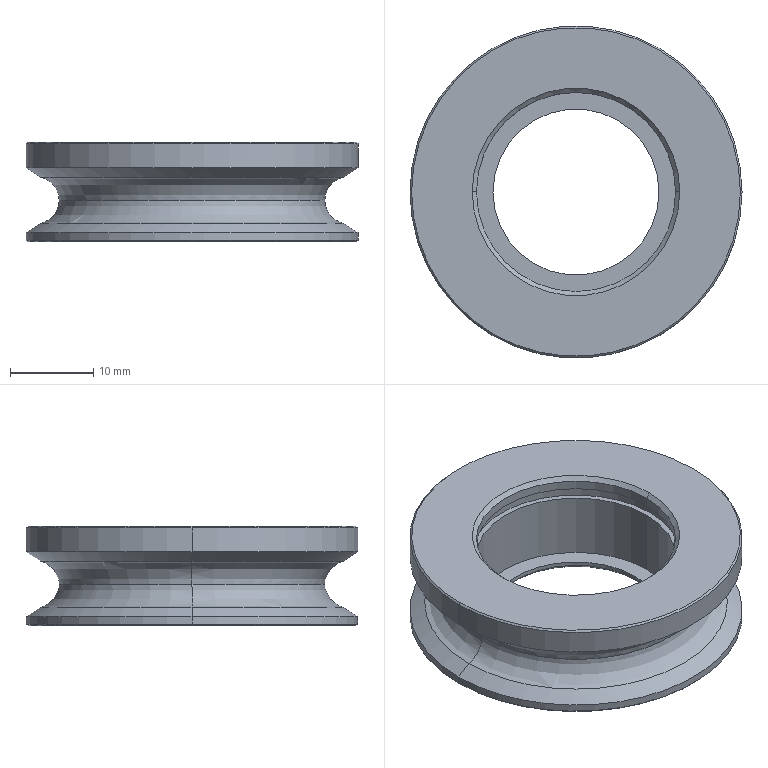Part | STEP file | 10000020541swp000-1 | 1 solid | 33 faces | box 40 x 40 x 12 mm | volume 7266 mm3 | cylinder 12 | cone 12 | plane 5 | torus 4 | commonest cylinder face diameters 24 x4 40 x4 20 x2 25.3 x2
STEP:
#1=CARTESIAN_POINT('',(12.65,0.,10.4));
#2=VERTEX_POINT('',#1);
#3=CARTESIAN_POINT('',(-12.65,0.,10.4));
#4=VERTEX_POINT('',#3);
#5=CARTESIAN_POINT('',(0.,0.,10.4));
#6=DIRECTION('',(0.,0.,-1.));
#7=DIRECTION('',(-1.,0.,0.));
#8=AXIS2_PLACEMENT_3D('',#5,#6,#7);
#9=CIRCLE('',#8,12.65);
#10=EDGE_CURVE('',#2,#4,#9,.T.);
#11=ORIENTED_EDGE('',*,*,#10,.F.);
#12=CARTESIAN_POINT('',(12.65,0.,9.));
#13=VERTEX_POINT('',#12);
#14=CARTESIAN_POINT('',(12.65,0.,0.));
#15=DIRECTION('',(0.,0.,-1.));
#16=VECTOR('',#15,1000.);
#17=LINE('',#14,#16);
#18=EDGE_CURVE('',#2,#13,#17,.T.);
#19=ORIENTED_EDGE('',*,*,#18,.T.);
#20=CARTESIAN_POINT('',(-12.65,0.,9.));
#21=VERTEX_POINT('',#20);
#22=CARTESIAN_POINT('',(0.,0.,9.));
#23=DIRECTION('',(0.,0.,-1.));
#24=DIRECTION('',(-1.,0.,0.));
#25=AXIS2_PLACEMENT_3D('',#22,#23,#24);
#26=CIRCLE('',#25,12.65);
#27=EDGE_CURVE('',#13,#21,#26,.T.);
#28=ORIENTED_EDGE('',*,*,#27,.T.);
#29=CARTESIAN_POINT('',(-12.65,0.,0.));
#30=DIRECTION('',(0.,0.,-1.));
#31=VECTOR('',#30,1000.);
#32=LINE('',#29,#31);
#33=EDGE_CURVE('',#4,#21,#32,.T.);
#34=ORIENTED_EDGE('',*,*,#33,.F.);
#35=EDGE_LOOP('',(#11,#19,#28,#34));
#36=FACE_OUTER_BOUND('',#35,.T.);
#37=CARTESIAN_POINT('',(0.,0.,0.));
#38=DIRECTION('',(0.,0.,-1.));
#39=DIRECTION('',(-1.,0.,0.));
#40=AXIS2_PLACEMENT_3D('',#37,#38,#39);
#41=CYLINDRICAL_SURFACE('',#40,12.65);
#42=ADVANCED_FACE('',(#36),#41,.F.);
#43=CARTESIAN_POINT('',(10.,0.,0.5));
#44=VERTEX_POINT('',#43);
#45=CARTESIAN_POINT('',(-10.,0.,0.5));
#46=VERTEX_POINT('',#45);
#47=CARTESIAN_POINT('',(0.,0.,0.5));
#48=DIRECTION('',(0.,0.,-1.));
#49=DIRECTION('',(1.,0.,0.));
#50=AXIS2_PLACEMENT_3D('',#47,#48,#49);
#51=CIRCLE('',#50,10.);
#52=EDGE_CURVE('',#44,#46,#51,.T.);
#53=ORIENTED_EDGE('',*,*,#52,.F.);
#54=CARTESIAN_POINT('',(10.5,0.,0.));
#55=VERTEX_POINT('',#54);
#56=CARTESIAN_POINT('',(10.5,0.,0.));
#57=DIRECTION('',(0.7071,0.,-0.7071));
#58=VECTOR('',#57,1000.);
#59=LINE('',#56,#58);
#60=EDGE_CURVE('',#44,#55,#59,.T.);
#61=ORIENTED_EDGE('',*,*,#60,.T.);
#62=CARTESIAN_POINT('',(-10.5,0.,0.));
#63=VERTEX_POINT('',#62);
#64=CARTESIAN_POINT('',(0.,0.,0.));
#65=DIRECTION('',(0.,0.,1.));
#66=DIRECTION('',(1.,0.,0.));
#67=AXIS2_PLACEMENT_3D('',#64,#65,#66);
#68=CIRCLE('',#67,10.5);
#69=EDGE_CURVE('',#63,#55,#68,.T.);
#70=ORIENTED_EDGE('',*,*,#69,.F.);
#71=CARTESIAN_POINT('',(-10.5,0.,0.));
#72=DIRECTION('',(-0.7071,0.,-0.7071));
#73=VECTOR('',#72,1000.);
#74=LINE('',#71,#73);
#75=EDGE_CURVE('',#46,#63,#74,.T.);
#76=ORIENTED_EDGE('',*,*,#75,.F.);
#77=EDGE_LOOP('',(#53,#61,#70,#76));
#78=FACE_OUTER_BOUND('',#77,.T.);
#79=CARTESIAN_POINT('',(0.,0.,0.));
#80=DIRECTION('',(0.,0.,-1.));
#81=DIRECTION('',(-1.,0.,0.));
#82=AXIS2_PLACEMENT_3D('',#79,#80,#81);
#83=CONICAL_SURFACE('',#82,10.5,0.7854);
#84=ADVANCED_FACE('',(#78),#83,.F.);
#85=CARTESIAN_POINT('',(-12.,0.,11.5));
#86=VERTEX_POINT('',#85);
#87=CARTESIAN_POINT('',(12.,0.,11.5));
#88=VERTEX_POINT('',#87);
#89=CARTESIAN_POINT('',(0.,0.,11.5));
#90=DIRECTION('',(0.,0.,1.));
#91=DIRECTION('',(1.,0.,0.));
#92=AXIS2_PLACEMENT_3D('',#89,#90,#91);
#93=CIRCLE('',#92,12.);
#94=EDGE_CURVE('',#86,#88,#93,.T.);
#95=ORIENTED_EDGE('',*,*,#94,.F.);
#96=CARTESIAN_POINT('',(-12.5,0.,12.));
#97=VERTEX_POINT('',#96);
#98=CARTESIAN_POINT('',(-12.,0.,11.5));
#99=DIRECTION('',(-0.7071,0.,0.7071));
#100=VECTOR('',#99,1000.);
#101=LINE('',#98,#100);
#102=EDGE_CURVE('',#86,#97,#101,.T.);
#103=ORIENTED_EDGE('',*,*,#102,.T.);
#104=CARTESIAN_POINT('',(12.5,0.,12.));
#105=VERTEX_POINT('',#104);
#106=CARTESIAN_POINT('',(0.,0.,12.));
#107=DIRECTION('',(0.,0.,-1.));
#108=DIRECTION('',(1.,0.,0.));
#109=AXIS2_PLACEMENT_3D('',#106,#107,#108);
#110=CIRCLE('',#109,12.5);
#111=EDGE_CURVE('',#105,#97,#110,.T.);
#112=ORIENTED_EDGE('',*,*,#111,.F.);
#113=CARTESIAN_POINT('',(12.,0.,11.5));
#114=DIRECTION('',(0.7071,0.,0.7071));
#115=VECTOR('',#114,1000.);
#116=LINE('',#113,#115);
#117=EDGE_CURVE('',#88,#105,#116,.T.);
#118=ORIENTED_EDGE('',*,*,#117,.F.);
#119=EDGE_LOOP('',(#95,#103,#112,#118));
#120=FACE_OUTER_BOUND('',#119,.T.);
#121=CARTESIAN_POINT('',(0.,0.,11.5));
#122=DIRECTION('',(0.,0.,1.));
#123=DIRECTION('',(1.,0.,0.));
#124=AXIS2_PLACEMENT_3D('',#121,#122,#123);
#125=CONICAL_SURFACE('',#124,12.,0.7854);
#126=ADVANCED_FACE('',(#120),#125,.F.);
#127=CARTESIAN_POINT('',(-19.8,0.,0.));
#128=VERTEX_POINT('',#127);
#129=CARTESIAN_POINT('',(19.8,0.,0.));
#130=VERTEX_POINT('',#129);
#131=CARTESIAN_POINT('',(0.,0.,0.));
#132=DIRECTION('',(0.,0.,-1.));
#133=DIRECTION('',(1.,0.,0.));
#134=AXIS2_PLACEMENT_3D('',#131,#132,#133);
#135=CIRCLE('',#134,19.8);
#136=EDGE_CURVE('',#128,#130,#135,.T.);
#137=ORIENTED_EDGE('',*,*,#136,.F.);
#138=CARTESIAN_POINT('',(-20.,0.,0.2));
#139=VERTEX_POINT('',#138);
#140=CARTESIAN_POINT('',(-20.,0.,0.2));
#141=DIRECTION('',(-0.7071,0.,0.7071));
#142=VECTOR('',#141,1000.);
#143=LINE('',#140,#142);
#144=EDGE_CURVE('',#128,#139,#143,.T.);
#145=ORIENTED_EDGE('',*,*,#144,.T.);
#146=CARTESIAN_POINT('',(20.,0.,0.2));
#147=VERTEX_POINT('',#146);
#148=CARTESIAN_POINT('',(0.,0.,0.2));
#149=DIRECTION('',(0.,0.,1.));
#150=DIRECTION('',(1.,0.,0.));
#151=AXIS2_PLACEMENT_3D('',#148,#149,#150);
#152=CIRCLE('',#151,20.);
#153=EDGE_CURVE('',#147,#139,#152,.T.);
#154=ORIENTED_EDGE('',*,*,#153,.F.);
#155=CARTESIAN_POINT('',(20.,0.,0.2));
#156=DIRECTION('',(0.7071,0.,0.7071));
#157=VECTOR('',#156,1000.);
#158=LINE('',#155,#157);
#159=EDGE_CURVE('',#130,#147,#158,.T.);
#160=ORIENTED_EDGE('',*,*,#159,.F.);
#161=EDGE_LOOP('',(#137,#145,#154,#160));
#162=FACE_OUTER_BOUND('',#161,.T.);
#163=CARTESIAN_POINT('',(0.,0.,0.2));
#164=DIRECTION('',(0.,0.,1.));
#165=DIRECTION('',(1.,0.,0.));
#166=AXIS2_PLACEMENT_3D('',#163,#164,#165);
#167=CONICAL_SURFACE('',#166,20.,0.7854);
#168=ADVANCED_FACE('',(#162),#167,.T.);
#169=CARTESIAN_POINT('',(19.8,0.,12.));
#170=VERTEX_POINT('',#169);
#171=CARTESIAN_POINT('',(-19.8,0.,12.));
#172=VERTEX_POINT('',#171);
#173=CARTESIAN_POINT('',(0.,0.,12.));
#174=DIRECTION('',(0.,0.,1.));
#175=DIRECTION('',(1.,0.,0.));
#176=AXIS2_PLACEMENT_3D('',#173,#174,#175);
#177=CIRCLE('',#176,19.8);
#178=EDGE_CURVE('',#170,#172,#177,.T.);
#179=ORIENTED_EDGE('',*,*,#178,.F.);
#180=CARTESIAN_POINT('',(20.,0.,11.8));
#181=VERTEX_POINT('',#180);
#182=CARTESIAN_POINT('',(19.8,0.,12.));
#183=DIRECTION('',(0.7071,0.,-0.7071));
#184=VECTOR('',#183,1000.);
#185=LINE('',#182,#184);
#186=EDGE_CURVE('',#170,#181,#185,.T.);
#187=ORIENTED_EDGE('',*,*,#186,.T.);
#188=CARTESIAN_POINT('',(-20.,0.,11.8));
#189=VERTEX_POINT('',#188);
#190=CARTESIAN_POINT('',(0.,0.,11.8));
#191=DIRECTION('',(0.,0.,-1.));
#192=DIRECTION('',(1.,0.,0.));
#193=AXIS2_PLACEMENT_3D('',#190,#191,#192);
#194=CIRCLE('',#193,20.);
#195=EDGE_CURVE('',#189,#181,#194,.T.);
#196=ORIENTED_EDGE('',*,*,#195,.F.);
#197=CARTESIAN_POINT('',(-19.8,0.,12.));
#198=DIRECTION('',(-0.7071,0.,-0.7071));
#199=VECTOR('',#198,1000.);
#200=LINE('',#197,#199);
#201=EDGE_CURVE('',#172,#189,#200,.T.);
#202=ORIENTED_EDGE('',*,*,#201,.F.);
#203=EDGE_LOOP('',(#179,#187,#196,#202));
#204=FACE_OUTER_BOUND('',#203,.T.);
#205=CARTESIAN_POINT('',(0.,0.,12.));
#206=DIRECTION('',(0.,0.,-1.));
#207=DIRECTION('',(-1.,0.,0.));
#208=AXIS2_PLACEMENT_3D('',#205,#206,#207);
#209=CONICAL_SURFACE('',#208,19.8,0.7854);
#210=ADVANCED_FACE('',(#204),#209,.T.);
#211=CARTESIAN_POINT('',(-18.244,0.,7.785));
#212=VERTEX_POINT('',#211);
#213=CARTESIAN_POINT('',(18.244,0.,7.785));
#214=VERTEX_POINT('',#213);
#215=CARTESIAN_POINT('',(0.,0.,7.785));
#216=DIRECTION('',(0.,0.,-1.));
#217=DIRECTION('',(-1.,0.,0.));
#218=AXIS2_PLACEMENT_3D('',#215,#216,#217);
#219=CIRCLE('',#218,18.244);
#220=EDGE_CURVE('',#212,#214,#219,.T.);
#221=ORIENTED_EDGE('',*,*,#220,.F.);
#222=CARTESIAN_POINT('',(-20.,0.,8.909));
#223=VERTEX_POINT('',#222);
#224=CARTESIAN_POINT('',(-20.,0.,8.909));
#225=DIRECTION('',(-0.8422,0.,0.5391));
#226=VECTOR('',#225,1000.);
#227=LINE('',#224,#226);
#228=EDGE_CURVE('',#212,#223,#227,.T.);
#229=ORIENTED_EDGE('',*,*,#228,.T.);
#230=CARTESIAN_POINT('',(20.,0.,8.909));
#231=VERTEX_POINT('',#230);
#232=CARTESIAN_POINT('',(0.,0.,8.909));
#233=DIRECTION('',(0.,0.,1.));
#234=DIRECTION('',(1.,0.,0.));
#235=AXIS2_PLACEMENT_3D('',#232,#233,#234);
#236=CIRCLE('',#235,20.);
#237=EDGE_CURVE('',#231,#223,#236,.T.);
#238=ORIENTED_EDGE('',*,*,#237,.F.);
#239=CARTESIAN_POINT('',(20.,0.,8.909));
#240=DIRECTION('',(0.8422,0.,0.5391));
#241=VECTOR('',#240,1000.);
#242=LINE('',#239,#241);
#243=EDGE_CURVE('',#214,#231,#242,.T.);
#244=ORIENTED_EDGE('',*,*,#243,.F.);
#245=EDGE_LOOP('',(#221,#229,#238,#244));
#246=FACE_OUTER_BOUND('',#245,.T.);
#247=CARTESIAN_POINT('',(0.,0.,8.909));
#248=DIRECTION('',(0.,0.,1.));
#249=DIRECTION('',(1.,0.,0.));
#250=AXIS2_PLACEMENT_3D('',#247,#248,#249);
#251=CONICAL_SURFACE('',#250,20.,1.001);
#252=ADVANCED_FACE('',(#246),#251,.T.);
#253=CARTESIAN_POINT('',(18.244,0.,2.215));
#254=VERTEX_POINT('',#253);
#255=CARTESIAN_POINT('',(-18.244,0.,2.215));
#256=VERTEX_POINT('',#255);
#257=CARTESIAN_POINT('',(0.,0.,2.215));
#258=DIRECTION('',(0.,0.,1.));
#259=DIRECTION('',(1.,0.,0.));
#260=AXIS2_PLACEMENT_3D('',#257,#258,#259);
#261=CIRCLE('',#260,18.244);
#262=EDGE_CURVE('',#254,#256,#261,.T.);
#263=ORIENTED_EDGE('',*,*,#262,.F.);
#264=CARTESIAN_POINT('',(20.,0.,1.091));
#265=VERTEX_POINT('',#264);
#266=CARTESIAN_POINT('',(18.244,0.,2.215));
#267=DIRECTION('',(0.8422,0.,-0.5391));
#268=VECTOR('',#267,1000.);
#269=LINE('',#266,#268);
#270=EDGE_CURVE('',#254,#265,#269,.T.);
#271=ORIENTED_EDGE('',*,*,#270,.T.);
#272=CARTESIAN_POINT('',(-20.,0.,1.091));
#273=VERTEX_POINT('',#272);
#274=CARTESIAN_POINT('',(0.,0.,1.091));
#275=DIRECTION('',(0.,0.,-1.));
#276=DIRECTION('',(-1.,0.,0.));
#277=AXIS2_PLACEMENT_3D('',#274,#275,#276);
#278=CIRCLE('',#277,20.);
#279=EDGE_CURVE('',#273,#265,#278,.T.);
#280=ORIENTED_EDGE('',*,*,#279,.F.);
#281=CARTESIAN_POINT('',(-18.244,0.,2.215));
#282=DIRECTION('',(-0.8422,0.,-0.5391));
#283=VECTOR('',#282,1000.);
#284=LINE('',#281,#283);
#285=EDGE_CURVE('',#256,#273,#284,.T.);
#286=ORIENTED_EDGE('',*,*,#285,.F.);
#287=EDGE_LOOP('',(#263,#271,#280,#286));
#288=FACE_OUTER_BOUND('',#287,.T.);
#289=CARTESIAN_POINT('',(0.,0.,2.215));
#290=DIRECTION('',(0.,0.,-1.));
#291=DIRECTION('',(-1.,0.,0.));
#292=AXIS2_PLACEMENT_3D('',#289,#290,#291);
#293=CONICAL_SURFACE('',#292,18.244,1.001);
#294=ADVANCED_FACE('',(#288),#293,.T.);
#295=CARTESIAN_POINT('',(0.,0.,2.215));
#296=DIRECTION('',(0.,0.,1.));
#297=DIRECTION('',(1.,0.,0.));
#298=AXIS2_PLACEMENT_3D('',#295,#296,#297);
#299=CIRCLE('',#298,18.244);
#300=EDGE_CURVE('',#256,#254,#299,.T.);
#301=ORIENTED_EDGE('',*,*,#300,.T.);
#302=CARTESIAN_POINT('',(16.,0.,5.));
#303=VERTEX_POINT('',#302);
#304=CARTESIAN_POINT('',(18.85,0.,5.));
#305=DIRECTION('',(0.,1.,0.));
#306=DIRECTION('',(-1.,0.,0.));
#307=AXIS2_PLACEMENT_3D('',#304,#305,#306);
#308=CIRCLE('',#307,2.85);
#309=EDGE_CURVE('',#254,#303,#308,.T.);
#310=ORIENTED_EDGE('',*,*,#309,.T.);
#311=CARTESIAN_POINT('',(-16.,0.,5.));
#312=VERTEX_POINT('',#311);
#313=CARTESIAN_POINT('',(0.,0.,5.));
#314=DIRECTION('',(0.,0.,-1.));
#315=DIRECTION('',(1.,0.,0.));
#316=AXIS2_PLACEMENT_3D('',#313,#314,#315);
#317=CIRCLE('',#316,16.);
#318=EDGE_CURVE('',#303,#312,#317,.T.);
#319=ORIENTED_EDGE('',*,*,#318,.T.);
#320=CARTESIAN_POINT('',(-18.85,0.,5.));
#321=DIRECTION('',(0.,-1.,0.));
#322=DIRECTION('',(0.,0.,-1.));
#323=AXIS2_PLACEMENT_3D('',#320,#321,#322);
#324=CIRCLE('',#323,2.85);
#325=EDGE_CURVE('',#256,#312,#324,.T.);
#326=ORIENTED_EDGE('',*,*,#325,.F.);
#327=EDGE_LOOP('',(#301,#310,#319,#326));
#328=FACE_OUTER_BOUND('',#327,.T.);
#329=CARTESIAN_POINT('',(0.,0.,5.));
#330=DIRECTION('',(0.,0.,-1.));
#331=DIRECTION('',(-1.,0.,0.));
#332=AXIS2_PLACEMENT_3D('',#329,#330,#331);
#333=TOROIDAL_SURFACE('',#332,18.85,2.85);
#334=ADVANCED_FACE('',(#328),#333,.F.);
#335=CARTESIAN_POINT('',(0.,0.,7.785));
#336=DIRECTION('',(0.,0.,-1.));
#337=DIRECTION('',(-1.,0.,0.));
#338=AXIS2_PLACEMENT_3D('',#335,#336,#337);
#339=CIRCLE('',#338,18.244);
#340=EDGE_CURVE('',#214,#212,#339,.T.);
#341=ORIENTED_EDGE('',*,*,#340,.T.);
#342=CARTESIAN_POINT('',(-18.85,0.,5.));
#343=DIRECTION('',(0.,1.,0.));
#344=DIRECTION('',(-1.,0.,0.));
#345=AXIS2_PLACEMENT_3D('',#342,#343,#344);
#346=CIRCLE('',#345,2.85);
#347=EDGE_CURVE('',#212,#312,#346,.T.);
#348=ORIENTED_EDGE('',*,*,#347,.T.);
#349=ORIENTED_EDGE('',*,*,#318,.F.);
#350=CARTESIAN_POINT('',(18.85,0.,5.));
#351=DIRECTION('',(0.,-1.,0.));
#352=DIRECTION('',(0.,0.,-1.));
#353=AXIS2_PLACEMENT_3D('',#350,#351,#352);
#354=CIRCLE('',#353,2.85);
#355=EDGE_CURVE('',#214,#303,#354,.T.);
#356=ORIENTED_EDGE('',*,*,#355,.F.);
#357=EDGE_LOOP('',(#341,#348,#349,#356));
#358=FACE_OUTER_BOUND('',#357,.T.);
#359=CARTESIAN_POINT('',(0.,0.,5.));
#360=DIRECTION('',(0.,0.,1.));
#361=DIRECTION('',(1.,0.,0.));
#362=AXIS2_PLACEMENT_3D('',#359,#360,#361);
#363=TOROIDAL_SURFACE('',#362,18.85,2.85);
#364=ADVANCED_FACE('',(#358),#363,.F.);
#365=CARTESIAN_POINT('',(-12.,0.,1.));
#366=VERTEX_POINT('',#365);
#367=CARTESIAN_POINT('',(12.,0.,1.));
#368=VERTEX_POINT('',#367);
#369=CARTESIAN_POINT('',(0.,0.,1.));
#370=DIRECTION('',(0.,0.,1.));
#371=DIRECTION('',(1.,0.,0.));
#372=AXIS2_PLACEMENT_3D('',#369,#370,#371);
#373=CIRCLE('',#372,12.);
#374=EDGE_CURVE('',#366,#368,#373,.T.);
#375=ORIENTED_EDGE('',*,*,#374,.F.);
#376=CARTESIAN_POINT('',(-12.,0.,9.));
#377=VERTEX_POINT('',#376);
#378=CARTESIAN_POINT('',(-12.,0.,1.));
#379=DIRECTION('',(0.,0.,1.));
#380=VECTOR('',#379,1000.);
#381=LINE('',#378,#380);
#382=EDGE_CURVE('',#366,#377,#381,.T.);
#383=ORIENTED_EDGE('',*,*,#382,.T.);
#384=CARTESIAN_POINT('',(12.,0.,9.));
#385=VERTEX_POINT('',#384);
#386=CARTESIAN_POINT('',(0.,0.,9.));
#387=DIRECTION('',(0.,0.,1.));
#388=DIRECTION('',(-1.,0.,0.));
#389=AXIS2_PLACEMENT_3D('',#386,#387,#388);
#390=CIRCLE('',#389,12.);
#391=EDGE_CURVE('',#377,#385,#390,.T.);
#392=ORIENTED_EDGE('',*,*,#391,.T.);
#393=CARTESIAN_POINT('',(12.,0.,1.));
#394=DIRECTION('',(0.,0.,1.));
#395=VECTOR('',#394,1000.);
#396=LINE('',#393,#395);
#397=EDGE_CURVE('',#368,#385,#396,.T.);
#398=ORIENTED_EDGE('',*,*,#397,.F.);
#399=EDGE_LOOP('',(#375,#383,#392,#398));
#400=FACE_OUTER_BOUND('',#399,.T.);
#401=CARTESIAN_POINT('',(0.,0.,1.));
#402=DIRECTION('',(0.,0.,1.));
#403=DIRECTION('',(1.,0.,0.));
#404=AXIS2_PLACEMENT_3D('',#401,#402,#403);
#405=CYLINDRICAL_SURFACE('',#404,12.);
#406=ADVANCED_FACE('',(#400),#405,.F.);
#407=ORIENTED_EDGE('',*,*,#279,.T.);
#408=CARTESIAN_POINT('',(20.,0.,12.));
#409=DIRECTION('',(0.,0.,-1.));
#410=VECTOR('',#409,1000.);
#411=LINE('',#408,#410);
#412=EDGE_CURVE('',#265,#147,#411,.T.);
#413=ORIENTED_EDGE('',*,*,#412,.T.);
#414=ORIENTED_EDGE('',*,*,#153,.T.);
#415=CARTESIAN_POINT('',(-20.,0.,12.));
#416=DIRECTION('',(0.,0.,-1.));
#417=VECTOR('',#416,1000.);
#418=LINE('',#415,#417);
#419=EDGE_CURVE('',#273,#139,#418,.T.);
#420=ORIENTED_EDGE('',*,*,#419,.F.);
#421=EDGE_LOOP('',(#407,#413,#414,#420));
#422=FACE_OUTER_BOUND('',#421,.T.);
#423=CARTESIAN_POINT('',(0.,0.,12.));
#424=DIRECTION('',(0.,0.,-1.));
#425=DIRECTION('',(-1.,0.,0.));
#426=AXIS2_PLACEMENT_3D('',#423,#424,#425);
#427=CYLINDRICAL_SURFACE('',#426,20.);
#428=ADVANCED_FACE('',(#422),#427,.T.);
#429=ORIENTED_EDGE('',*,*,#195,.T.);
#430=CARTESIAN_POINT('',(20.,0.,12.));
#431=DIRECTION('',(0.,0.,-1.));
#432=VECTOR('',#431,1000.);
#433=LINE('',#430,#432);
#434=EDGE_CURVE('',#181,#231,#433,.T.);
#435=ORIENTED_EDGE('',*,*,#434,.T.);
#436=ORIENTED_EDGE('',*,*,#237,.T.);
#437=CARTESIAN_POINT('',(-20.,0.,12.));
#438=DIRECTION('',(0.,0.,-1.));
#439=VECTOR('',#438,1000.);
#440=LINE('',#437,#439);
#441=EDGE_CURVE('',#189,#223,#440,.T.);
#442=ORIENTED_EDGE('',*,*,#441,.F.);
#443=EDGE_LOOP('',(#429,#435,#436,#442));
#444=FACE_OUTER_BOUND('',#443,.T.);
#445=CARTESIAN_POINT('',(0.,0.,12.));
#446=DIRECTION('',(0.,0.,-1.));
#447=DIRECTION('',(-1.,0.,0.));
#448=AXIS2_PLACEMENT_3D('',#445,#446,#447);
#449=CYLINDRICAL_SURFACE('',#448,20.);
#450=ADVANCED_FACE('',(#444),#449,.T.);
#451=ORIENTED_EDGE('',*,*,#52,.T.);
#452=CARTESIAN_POINT('',(-10.,0.,1.));
#453=VERTEX_POINT('',#452);
#454=CARTESIAN_POINT('',(-10.,0.,12.));
#455=DIRECTION('',(0.,0.,1.));
#456=VECTOR('',#455,1000.);
#457=LINE('',#454,#456);
#458=EDGE_CURVE('',#46,#453,#457,.T.);
#459=ORIENTED_EDGE('',*,*,#458,.T.);
#460=CARTESIAN_POINT('',(10.,0.,1.));
#461=VERTEX_POINT('',#460);
#462=CARTESIAN_POINT('',(0.,0.,1.));
#463=DIRECTION('',(0.,0.,-1.));
#464=DIRECTION('',(1.,0.,0.));
#465=AXIS2_PLACEMENT_3D('',#462,#463,#464);
#466=CIRCLE('',#465,10.);
#467=EDGE_CURVE('',#461,#453,#466,.T.);
#468=ORIENTED_EDGE('',*,*,#467,.F.);
#469=CARTESIAN_POINT('',(10.,0.,12.));
#470=DIRECTION('',(0.,0.,1.));
#471=VECTOR('',#470,1000.);
#472=LINE('',#469,#471);
#473=EDGE_CURVE('',#44,#461,#472,.T.);
#474=ORIENTED_EDGE('',*,*,#473,.F.);
#475=EDGE_LOOP('',(#451,#459,#468,#474));
#476=FACE_OUTER_BOUND('',#475,.T.);
#477=CARTESIAN_POINT('',(0.,0.,12.));
#478=DIRECTION('',(0.,0.,1.));
#479=DIRECTION('',(1.,0.,0.));
#480=AXIS2_PLACEMENT_3D('',#477,#478,#479);
#481=CYLINDRICAL_SURFACE('',#480,10.);
#482=ADVANCED_FACE('',(#476),#481,.F.);
#483=CARTESIAN_POINT('',(12.,0.,10.4));
#484=VERTEX_POINT('',#483);
#485=CARTESIAN_POINT('',(-12.,0.,10.4));
#486=VERTEX_POINT('',#485);
#487=CARTESIAN_POINT('',(0.,0.,10.4));
#488=DIRECTION('',(0.,0.,-1.));
#489=DIRECTION('',(1.,0.,0.));
#490=AXIS2_PLACEMENT_3D('',#487,#488,#489);
#491=CIRCLE('',#490,12.);
#492=EDGE_CURVE('',#484,#486,#491,.T.);
#493=ORIENTED_EDGE('',*,*,#492,.T.);
#494=CARTESIAN_POINT('',(-12.,0.,1.));
#495=DIRECTION('',(0.,0.,1.));
#496=VECTOR('',#495,1000.);
#497=LINE('',#494,#496);
#498=EDGE_CURVE('',#486,#86,#497,.T.);
#499=ORIENTED_EDGE('',*,*,#498,.T.);
#500=ORIENTED_EDGE('',*,*,#94,.T.);
#501=CARTESIAN_POINT('',(12.,0.,1.));
#502=DIRECTION('',(0.,0.,1.));
#503=VECTOR('',#502,1000.);
#504=LINE('',#501,#503);
#505=EDGE_CURVE('',#484,#88,#504,.T.);
#506=ORIENTED_EDGE('',*,*,#505,.F.);
#507=EDGE_LOOP('',(#493,#499,#500,#506));
#508=FACE_OUTER_BOUND('',#507,.T.);
#509=CARTESIAN_POINT('',(0.,0.,1.));
#510=DIRECTION('',(0.,0.,1.));
#511=DIRECTION('',(1.,0.,0.));
#512=AXIS2_PLACEMENT_3D('',#509,#510,#511);
#513=CYLINDRICAL_SURFACE('',#512,12.);
#514=ADVANCED_FACE('',(#508),#513,.F.);
#515=ORIENTED_EDGE('',*,*,#498,.F.);
#516=CARTESIAN_POINT('',(0.,0.,10.4));
#517=DIRECTION('',(0.,0.,-1.));
#518=DIRECTION('',(1.,0.,0.));
#519=AXIS2_PLACEMENT_3D('',#516,#517,#518);
#520=CIRCLE('',#519,12.);
#521=EDGE_CURVE('',#486,#484,#520,.T.);
#522=ORIENTED_EDGE('',*,*,#521,.T.);
#523=ORIENTED_EDGE('',*,*,#505,.T.);
#524=CARTESIAN_POINT('',(0.,0.,11.5));
#525=DIRECTION('',(0.,0.,1.));
#526=DIRECTION('',(1.,0.,0.));
#527=AXIS2_PLACEMENT_3D('',#524,#525,#526);
#528=CIRCLE('',#527,12.);
#529=EDGE_CURVE('',#88,#86,#528,.T.);
#530=ORIENTED_EDGE('',*,*,#529,.T.);
#531=EDGE_LOOP('',(#515,#522,#523,#530));
#532=FACE_OUTER_BOUND('',#531,.T.);
#533=CARTESIAN_POINT('',(0.,0.,1.));
#534=DIRECTION('',(0.,0.,1.));
#535=DIRECTION('',(1.,0.,0.));
#536=AXIS2_PLACEMENT_3D('',#533,#534,#535);
#537=CYLINDRICAL_SURFACE('',#536,12.);
#538=ADVANCED_FACE('',(#532),#537,.F.);
#539=ORIENTED_EDGE('',*,*,#458,.F.);
#540=CARTESIAN_POINT('',(0.,0.,0.5));
#541=DIRECTION('',(0.,0.,-1.));
#542=DIRECTION('',(1.,0.,0.));
#543=AXIS2_PLACEMENT_3D('',#540,#541,#542);
#544=CIRCLE('',#543,10.);
#545=EDGE_CURVE('',#46,#44,#544,.T.);
#546=ORIENTED_EDGE('',*,*,#545,.T.);
#547=ORIENTED_EDGE('',*,*,#473,.T.);
#548=CARTESIAN_POINT('',(0.,0.,1.));
#549=DIRECTION('',(0.,0.,-1.));
#550=DIRECTION('',(1.,0.,0.));
#551=AXIS2_PLACEMENT_3D('',#548,#549,#550);
#552=CIRCLE('',#551,10.);
#553=EDGE_CURVE('',#453,#461,#552,.T.);
#554=ORIENTED_EDGE('',*,*,#553,.F.);
#555=EDGE_LOOP('',(#539,#546,#547,#554));
#556=FACE_OUTER_BOUND('',#555,.T.);
#557=CARTESIAN_POINT('',(0.,0.,12.));
#558=DIRECTION('',(0.,0.,1.));
#559=DIRECTION('',(1.,0.,0.));
#560=AXIS2_PLACEMENT_3D('',#557,#558,#559);
#561=CYLINDRICAL_SURFACE('',#560,10.);
#562=ADVANCED_FACE('',(#556),#561,.F.);
#563=ORIENTED_EDGE('',*,*,#434,.F.);
#564=CARTESIAN_POINT('',(0.,0.,11.8));
#565=DIRECTION('',(0.,0.,-1.));
#566=DIRECTION('',(1.,0.,0.));
#567=AXIS2_PLACEMENT_3D('',#564,#565,#566);
#568=CIRCLE('',#567,20.);
#569=EDGE_CURVE('',#181,#189,#568,.T.);
#570=ORIENTED_EDGE('',*,*,#569,.T.);
#571=ORIENTED_EDGE('',*,*,#441,.T.);
#572=CARTESIAN_POINT('',(0.,0.,8.909));
#573=DIRECTION('',(0.,0.,1.));
#574=DIRECTION('',(1.,0.,0.));
#575=AXIS2_PLACEMENT_3D('',#572,#573,#574);
#576=CIRCLE('',#575,20.);
#577=EDGE_CURVE('',#223,#231,#576,.T.);
#578=ORIENTED_EDGE('',*,*,#577,.T.);
#579=EDGE_LOOP('',(#563,#570,#571,#578));
#580=FACE_OUTER_BOUND('',#579,.T.);
#581=CARTESIAN_POINT('',(0.,0.,12.));
#582=DIRECTION('',(0.,0.,-1.));
#583=DIRECTION('',(-1.,0.,0.));
#584=AXIS2_PLACEMENT_3D('',#581,#582,#583);
#585=CYLINDRICAL_SURFACE('',#584,20.);
#586=ADVANCED_FACE('',(#580),#585,.T.);
#587=ORIENTED_EDGE('',*,*,#412,.F.);
#588=CARTESIAN_POINT('',(0.,0.,1.091));
#589=DIRECTION('',(0.,0.,-1.));
#590=DIRECTION('',(-1.,0.,0.));
#591=AXIS2_PLACEMENT_3D('',#588,#589,#590);
#592=CIRCLE('',#591,20.);
#593=EDGE_CURVE('',#265,#273,#592,.T.);
#594=ORIENTED_EDGE('',*,*,#593,.T.);
#595=ORIENTED_EDGE('',*,*,#419,.T.);
#596=CARTESIAN_POINT('',(0.,0.,0.2));
#597=DIRECTION('',(0.,0.,1.));
#598=DIRECTION('',(1.,0.,0.));
#599=AXIS2_PLACEMENT_3D('',#596,#597,#598);
#600=CIRCLE('',#599,20.);
#601=EDGE_CURVE('',#139,#147,#600,.T.);
#602=ORIENTED_EDGE('',*,*,#601,.T.);
#603=EDGE_LOOP('',(#587,#594,#595,#602));
#604=FACE_OUTER_BOUND('',#603,.T.);
#605=CARTESIAN_POINT('',(0.,0.,12.));
#606=DIRECTION('',(0.,0.,-1.));
#607=DIRECTION('',(-1.,0.,0.));
#608=AXIS2_PLACEMENT_3D('',#605,#606,#607);
#609=CYLINDRICAL_SURFACE('',#608,20.);
#610=ADVANCED_FACE('',(#604),#609,.T.);
#611=ORIENTED_EDGE('',*,*,#111,.T.);
#612=CARTESIAN_POINT('',(0.,0.,12.));
#613=DIRECTION('',(0.,0.,-1.));
#614=DIRECTION('',(1.,0.,0.));
#615=AXIS2_PLACEMENT_3D('',#612,#613,#614);
#616=CIRCLE('',#615,12.5);
#617=EDGE_CURVE('',#97,#105,#616,.T.);
#618=ORIENTED_EDGE('',*,*,#617,.T.);
#619=EDGE_LOOP('',(#611,#618));
#620=FACE_BOUND('',#619,.T.);
#621=CARTESIAN_POINT('',(0.,0.,12.));
#622=DIRECTION('',(0.,0.,1.));
#623=DIRECTION('',(1.,0.,0.));
#624=AXIS2_PLACEMENT_3D('',#621,#622,#623);
#625=CIRCLE('',#624,19.8);
#626=EDGE_CURVE('',#172,#170,#625,.T.);
#627=ORIENTED_EDGE('',*,*,#626,.T.);
#628=ORIENTED_EDGE('',*,*,#178,.T.);
#629=EDGE_LOOP('',(#627,#628));
#630=FACE_OUTER_BOUND('',#629,.T.);
#631=CARTESIAN_POINT('',(0.,0.,12.));
#632=DIRECTION('',(0.,0.,1.));
#633=DIRECTION('',(1.,0.,0.));
#634=AXIS2_PLACEMENT_3D('',#631,#632,#633);
#635=PLANE('',#634);
#636=ADVANCED_FACE('',(#620,#630),#635,.T.);
#637=ORIENTED_EDGE('',*,*,#69,.T.);
#638=CARTESIAN_POINT('',(0.,0.,0.));
#639=DIRECTION('',(0.,0.,1.));
#640=DIRECTION('',(1.,0.,0.));
#641=AXIS2_PLACEMENT_3D('',#638,#639,#640);
#642=CIRCLE('',#641,10.5);
#643=EDGE_CURVE('',#55,#63,#642,.T.);
#644=ORIENTED_EDGE('',*,*,#643,.T.);
#645=EDGE_LOOP('',(#637,#644));
#646=FACE_BOUND('',#645,.T.);
#647=CARTESIAN_POINT('',(0.,0.,0.));
#648=DIRECTION('',(0.,0.,-1.));
#649=DIRECTION('',(1.,0.,0.));
#650=AXIS2_PLACEMENT_3D('',#647,#648,#649);
#651=CIRCLE('',#650,19.8);
#652=EDGE_CURVE('',#130,#128,#651,.T.);
#653=ORIENTED_EDGE('',*,*,#652,.T.);
#654=ORIENTED_EDGE('',*,*,#136,.T.);
#655=EDGE_LOOP('',(#653,#654));
#656=FACE_OUTER_BOUND('',#655,.T.);
#657=CARTESIAN_POINT('',(0.,0.,0.));
#658=DIRECTION('',(0.,0.,1.));
#659=DIRECTION('',(1.,0.,0.));
#660=AXIS2_PLACEMENT_3D('',#657,#658,#659);
#661=PLANE('',#660);
#662=ADVANCED_FACE('',(#646,#656),#661,.F.);
#663=CARTESIAN_POINT('',(0.,0.,1.));
#664=DIRECTION('',(0.,0.,1.));
#665=DIRECTION('',(1.,0.,0.));
#666=AXIS2_PLACEMENT_3D('',#663,#664,#665);
#667=CIRCLE('',#666,12.);
#668=EDGE_CURVE('',#368,#366,#667,.T.);
#669=ORIENTED_EDGE('',*,*,#668,.T.);
#670=ORIENTED_EDGE('',*,*,#374,.T.);
#671=EDGE_LOOP('',(#669,#670));
#672=FACE_OUTER_BOUND('',#671,.T.);
#673=ORIENTED_EDGE('',*,*,#467,.T.);
#674=ORIENTED_EDGE('',*,*,#553,.T.);
#675=EDGE_LOOP('',(#673,#674));
#676=FACE_BOUND('',#675,.T.);
#677=CARTESIAN_POINT('',(0.,0.,1.));
#678=DIRECTION('',(0.,0.,1.));
#679=DIRECTION('',(1.,0.,0.));
#680=AXIS2_PLACEMENT_3D('',#677,#678,#679);
#681=PLANE('',#680);
#682=ADVANCED_FACE('',(#672,#676),#681,.T.);
#683=ORIENTED_EDGE('',*,*,#382,.F.);
#684=ORIENTED_EDGE('',*,*,#668,.F.);
#685=ORIENTED_EDGE('',*,*,#397,.T.);
#686=CARTESIAN_POINT('',(0.,0.,9.));
#687=DIRECTION('',(0.,0.,1.));
#688=DIRECTION('',(-1.,0.,0.));
#689=AXIS2_PLACEMENT_3D('',#686,#687,#688);
#690=CIRCLE('',#689,12.);
#691=EDGE_CURVE('',#385,#377,#690,.T.);
#692=ORIENTED_EDGE('',*,*,#691,.T.);
#693=EDGE_LOOP('',(#683,#684,#685,#692));
#694=FACE_OUTER_BOUND('',#693,.T.);
#695=CARTESIAN_POINT('',(0.,0.,1.));
#696=DIRECTION('',(0.,0.,1.));
#697=DIRECTION('',(1.,0.,0.));
#698=AXIS2_PLACEMENT_3D('',#695,#696,#697);
#699=CYLINDRICAL_SURFACE('',#698,12.);
#700=ADVANCED_FACE('',(#694),#699,.F.);
#701=ORIENTED_EDGE('',*,*,#347,.F.);
#702=ORIENTED_EDGE('',*,*,#220,.T.);
#703=ORIENTED_EDGE('',*,*,#355,.T.);
#704=CARTESIAN_POINT('',(0.,0.,5.));
#705=DIRECTION('',(0.,0.,-1.));
#706=DIRECTION('',(1.,0.,0.));
#707=AXIS2_PLACEMENT_3D('',#704,#705,#706);
#708=CIRCLE('',#707,16.);
#709=EDGE_CURVE('',#312,#303,#708,.T.);
#710=ORIENTED_EDGE('',*,*,#709,.F.);
#711=EDGE_LOOP('',(#701,#702,#703,#710));
#712=FACE_OUTER_BOUND('',#711,.T.);
#713=CARTESIAN_POINT('',(0.,0.,5.));
#714=DIRECTION('',(0.,0.,1.));
#715=DIRECTION('',(1.,0.,0.));
#716=AXIS2_PLACEMENT_3D('',#713,#714,#715);
#717=TOROIDAL_SURFACE('',#716,18.85,2.85);
#718=ADVANCED_FACE('',(#712),#717,.F.);
#719=ORIENTED_EDGE('',*,*,#309,.F.);
#720=ORIENTED_EDGE('',*,*,#262,.T.);
#721=ORIENTED_EDGE('',*,*,#325,.T.);
#722=ORIENTED_EDGE('',*,*,#709,.T.);
#723=EDGE_LOOP('',(#719,#720,#721,#722));
#724=FACE_OUTER_BOUND('',#723,.T.);
#725=CARTESIAN_POINT('',(0.,0.,5.));
#726=DIRECTION('',(0.,0.,-1.));
#727=DIRECTION('',(-1.,0.,0.));
#728=AXIS2_PLACEMENT_3D('',#725,#726,#727);
#729=TOROIDAL_SURFACE('',#728,18.85,2.85);
#730=ADVANCED_FACE('',(#724),#729,.F.);
#731=ORIENTED_EDGE('',*,*,#270,.F.);
#732=ORIENTED_EDGE('',*,*,#300,.F.);
#733=ORIENTED_EDGE('',*,*,#285,.T.);
#734=ORIENTED_EDGE('',*,*,#593,.F.);
#735=EDGE_LOOP('',(#731,#732,#733,#734));
#736=FACE_OUTER_BOUND('',#735,.T.);
#737=CARTESIAN_POINT('',(0.,0.,2.215));
#738=DIRECTION('',(0.,0.,-1.));
#739=DIRECTION('',(-1.,0.,0.));
#740=AXIS2_PLACEMENT_3D('',#737,#738,#739);
#741=CONICAL_SURFACE('',#740,18.244,1.001);
#742=ADVANCED_FACE('',(#736),#741,.T.);
#743=ORIENTED_EDGE('',*,*,#228,.F.);
#744=ORIENTED_EDGE('',*,*,#340,.F.);
#745=ORIENTED_EDGE('',*,*,#243,.T.);
#746=ORIENTED_EDGE('',*,*,#577,.F.);
#747=EDGE_LOOP('',(#743,#744,#745,#746));
#748=FACE_OUTER_BOUND('',#747,.T.);
#749=CARTESIAN_POINT('',(0.,0.,8.909));
#750=DIRECTION('',(0.,0.,1.));
#751=DIRECTION('',(1.,0.,0.));
#752=AXIS2_PLACEMENT_3D('',#749,#750,#751);
#753=CONICAL_SURFACE('',#752,20.,1.001);
#754=ADVANCED_FACE('',(#748),#753,.T.);
#755=ORIENTED_EDGE('',*,*,#186,.F.);
#756=ORIENTED_EDGE('',*,*,#626,.F.);
#757=ORIENTED_EDGE('',*,*,#201,.T.);
#758=ORIENTED_EDGE('',*,*,#569,.F.);
#759=EDGE_LOOP('',(#755,#756,#757,#758));
#760=FACE_OUTER_BOUND('',#759,.T.);
#761=CARTESIAN_POINT('',(0.,0.,12.));
#762=DIRECTION('',(0.,0.,-1.));
#763=DIRECTION('',(-1.,0.,0.));
#764=AXIS2_PLACEMENT_3D('',#761,#762,#763);
#765=CONICAL_SURFACE('',#764,19.8,0.7854);
#766=ADVANCED_FACE('',(#760),#765,.T.);
#767=ORIENTED_EDGE('',*,*,#144,.F.);
#768=ORIENTED_EDGE('',*,*,#652,.F.);
#769=ORIENTED_EDGE('',*,*,#159,.T.);
#770=ORIENTED_EDGE('',*,*,#601,.F.);
#771=EDGE_LOOP('',(#767,#768,#769,#770));
#772=FACE_OUTER_BOUND('',#771,.T.);
#773=CARTESIAN_POINT('',(0.,0.,0.2));
#774=DIRECTION('',(0.,0.,1.));
#775=DIRECTION('',(1.,0.,0.));
#776=AXIS2_PLACEMENT_3D('',#773,#774,#775);
#777=CONICAL_SURFACE('',#776,20.,0.7854);
#778=ADVANCED_FACE('',(#772),#777,.T.);
#779=ORIENTED_EDGE('',*,*,#102,.F.);
#780=ORIENTED_EDGE('',*,*,#529,.F.);
#781=ORIENTED_EDGE('',*,*,#117,.T.);
#782=ORIENTED_EDGE('',*,*,#617,.F.);
#783=EDGE_LOOP('',(#779,#780,#781,#782));
#784=FACE_OUTER_BOUND('',#783,.T.);
#785=CARTESIAN_POINT('',(0.,0.,11.5));
#786=DIRECTION('',(0.,0.,1.));
#787=DIRECTION('',(1.,0.,0.));
#788=AXIS2_PLACEMENT_3D('',#785,#786,#787);
#789=CONICAL_SURFACE('',#788,12.,0.7854);
#790=ADVANCED_FACE('',(#784),#789,.F.);
#791=ORIENTED_EDGE('',*,*,#60,.F.);
#792=ORIENTED_EDGE('',*,*,#545,.F.);
#793=ORIENTED_EDGE('',*,*,#75,.T.);
#794=ORIENTED_EDGE('',*,*,#643,.F.);
#795=EDGE_LOOP('',(#791,#792,#793,#794));
#796=FACE_OUTER_BOUND('',#795,.T.);
#797=CARTESIAN_POINT('',(0.,0.,0.));
#798=DIRECTION('',(0.,0.,-1.));
#799=DIRECTION('',(-1.,0.,0.));
#800=AXIS2_PLACEMENT_3D('',#797,#798,#799);
#801=CONICAL_SURFACE('',#800,10.5,0.7854);
#802=ADVANCED_FACE('',(#796),#801,.F.);
#803=CARTESIAN_POINT('',(0.,0.,10.4));
#804=DIRECTION('',(0.,0.,-1.));
#805=DIRECTION('',(-1.,0.,0.));
#806=AXIS2_PLACEMENT_3D('',#803,#804,#805);
#807=CIRCLE('',#806,12.65);
#808=EDGE_CURVE('',#4,#2,#807,.T.);
#809=ORIENTED_EDGE('',*,*,#808,.T.);
#810=ORIENTED_EDGE('',*,*,#10,.T.);
#811=EDGE_LOOP('',(#809,#810));
#812=FACE_OUTER_BOUND('',#811,.T.);
#813=ORIENTED_EDGE('',*,*,#492,.F.);
#814=ORIENTED_EDGE('',*,*,#521,.F.);
#815=EDGE_LOOP('',(#813,#814));
#816=FACE_BOUND('',#815,.T.);
#817=CARTESIAN_POINT('',(-11.345,0.,10.4));
#818=DIRECTION('',(0.,0.,1.));
#819=DIRECTION('',(1.,0.,0.));
#820=AXIS2_PLACEMENT_3D('',#817,#818,#819);
#821=PLANE('',#820);
#822=ADVANCED_FACE('',(#812,#816),#821,.F.);
#823=CARTESIAN_POINT('',(0.,0.,9.));
#824=DIRECTION('',(0.,0.,-1.));
#825=DIRECTION('',(-1.,0.,0.));
#826=AXIS2_PLACEMENT_3D('',#823,#824,#825);
#827=CIRCLE('',#826,12.65);
#828=EDGE_CURVE('',#21,#13,#827,.T.);
#829=ORIENTED_EDGE('',*,*,#828,.F.);
#830=ORIENTED_EDGE('',*,*,#27,.F.);
#831=EDGE_LOOP('',(#829,#830));
#832=FACE_OUTER_BOUND('',#831,.T.);
#833=ORIENTED_EDGE('',*,*,#691,.F.);
#834=ORIENTED_EDGE('',*,*,#391,.F.);
#835=EDGE_LOOP('',(#833,#834));
#836=FACE_BOUND('',#835,.T.);
#837=CARTESIAN_POINT('',(-11.345,0.,9.));
#838=DIRECTION('',(0.,0.,-1.));
#839=DIRECTION('',(-1.,0.,0.));
#840=AXIS2_PLACEMENT_3D('',#837,#838,#839);
#841=PLANE('',#840);
#842=ADVANCED_FACE('',(#832,#836),#841,.F.);
#843=ORIENTED_EDGE('',*,*,#18,.F.);
#844=ORIENTED_EDGE('',*,*,#808,.F.);
#845=ORIENTED_EDGE('',*,*,#33,.T.);
#846=ORIENTED_EDGE('',*,*,#828,.T.);
#847=EDGE_LOOP('',(#843,#844,#845,#846));
#848=FACE_OUTER_BOUND('',#847,.T.);
#849=CARTESIAN_POINT('',(0.,0.,0.));
#850=DIRECTION('',(0.,0.,-1.));
#851=DIRECTION('',(-1.,0.,0.));
#852=AXIS2_PLACEMENT_3D('',#849,#850,#851);
#853=CYLINDRICAL_SURFACE('',#852,12.65);
#854=ADVANCED_FACE('',(#848),#853,.F.);
#855=CLOSED_SHELL('',(#42,#84,#126,#168,#210,#252,#294,#334,#364,#406,#428,#450,#482,#514,#538,#562,#586,#610,#636,#662,#682,#700,#718,#730,#742,#754,#766,#778,#790,#802,#822,#842,#854));
#856=MANIFOLD_SOLID_BREP('',#855);
#857=CARTESIAN_POINT('',(0.,0.,0.));
#858=DIRECTION('',(0.,0.,1.));
#859=DIRECTION('',(1.,0.,0.));
#860=AXIS2_PLACEMENT_3D('',#857,#858,#859);
#861=(LENGTH_UNIT()NAMED_UNIT(*)SI_UNIT(.MILLI.,.METRE.));
#862=UNCERTAINTY_MEASURE_WITH_UNIT(LENGTH_MEASURE(0.00001),#861,'','');
#863=(NAMED_UNIT(*)PLANE_ANGLE_UNIT()SI_UNIT($,.RADIAN.));
#864=(NAMED_UNIT(*)SI_UNIT($,.STERADIAN.)SOLID_ANGLE_UNIT());
#865=(GEOMETRIC_REPRESENTATION_CONTEXT(3)GLOBAL_UNCERTAINTY_ASSIGNED_CONTEXT((#862))GLOBAL_UNIT_ASSIGNED_CONTEXT((#861,#863,#864))REPRESENTATION_CONTEXT('',''));
#866=ADVANCED_BREP_SHAPE_REPRESENTATION('',(#856,#860),#865);